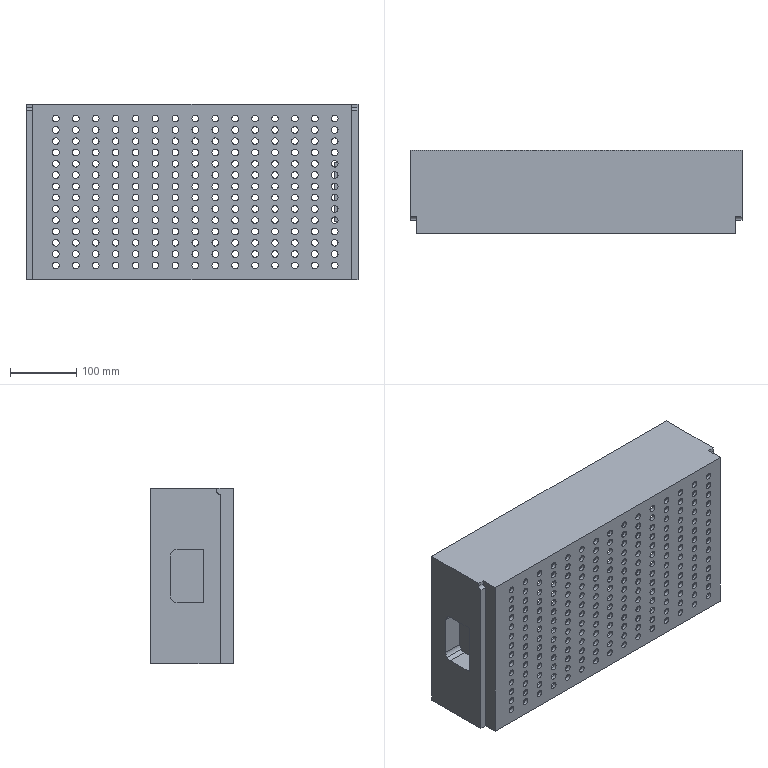Part | SolidWorks | features BaseBody 1 | 1 solid | 481 faces | box 500 x 125 x 265 mm | volume 1562536 mm3 | cylinder 440 | plane 41 | commonest cylinder face diameters 10 x422 20 x10 30 x8